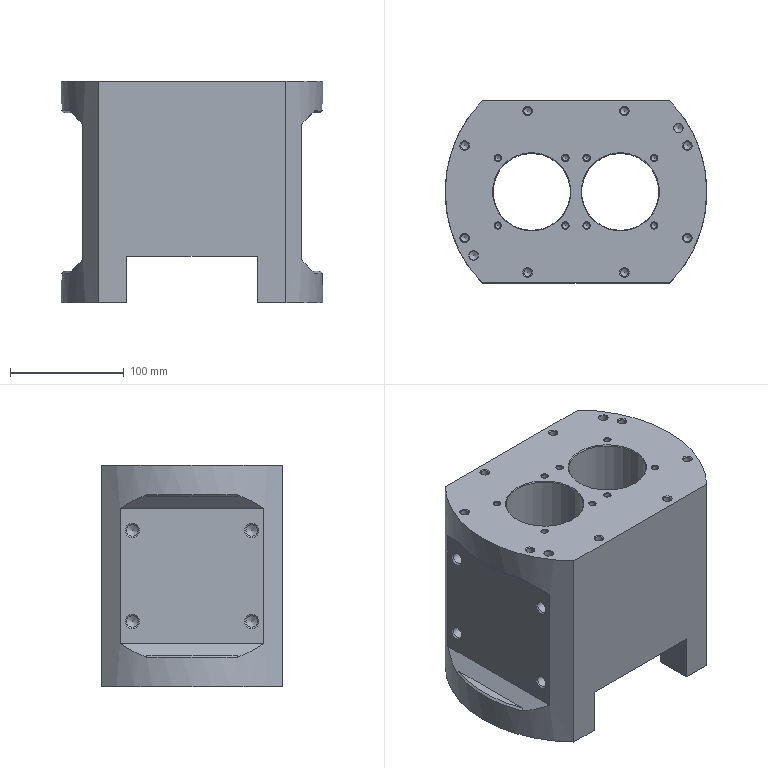CAM job | NX | 3+2 milling, drilling | part box 230 x 160 x 195 mm | stock box 230 x 230 x 195 mm
Tools:
number,name,description,diameter,corner_radius,flute_length,length,flutes
2,D50,Milling Tool-5 Parameters,50.0,0.0,50.0,75.0,2
1,ZXZ,Milling Tool-5 Parameters,6.0,0.0,50.0,75.0,2
11,10.2ZT,Drilling Tool,10.2,0.0,35.0,50.0,2
12,M12,Milling Tool-5 Parameters,10.2,0.0,30.0,30.0,4
7,D6A45,Milling Tool-5 Parameters,6.0,0.0,50.0,75.0,2
5,D6R0.5,Milling Tool-5 Parameters,6.0,0.5,50.0,75.0,2
10,D10,Milling Tool-5 Parameters,10.0,0.0,50.0,75.0,2
16,6.8ZT,Drilling Tool,6.8,0.0,35.0,50.0,2
18,M8,Milling Tool-5 Parameters,6.8,0.0,30.0,30.0,4
15,5.2ZT,Drilling Tool,5.0,0.0,35.0,50.0,2
14,M6,Milling Tool-5 Parameters,5.0,0.0,30.0,30.0,4
17,7.8ZT,Drilling Tool,7.8,0.0,35.0,50.0,2
18,8.0JD,Milling Tool-5 Parameters,8.0,0.0,30.0,30.0,4
19,11.8ZT,Drilling Tool,11.8,0.0,35.0,50.0,2
9,D35R.5,Milling Tool-5 Parameters,35.0,0.5,50.0,75.0,2
8,68.0JD,Milling Tool-5 Parameters,68.0,0.0,50.0,75.0,2
11,D10JING,Milling Tool-5 Parameters,10.0,0.0,50.0,75.0,2
20,8.5ZT,Drilling Tool,8.5,0.0,35.0,50.0,2
21,M10,Milling Tool-5 Parameters,8.5,0.0,30.0,30.0,4
22,12.0JD,Milling Tool-5 Parameters,12.0,0.0,30.0,30.0,4
Operations:
program,operation,operation_type,tool,method,geometry_group,spindle_rpm,surface_speed,feed_per_tooth,feed_cut,feed_plunge,cut_length_mm,path_length_mm,cut_time_min,machine_time_min
1,FLOOR_WALL,VolumeBased25DMillingOperation,D50,METHOD,A,1200.0,188.0,0.8333,2000.0,1000.0,131491.296,159721.141,66.046,68.869
1,FLOOR_WALL_COPY,VolumeBased25DMillingOperation,D50,METHOD,A,2500.0,392.0,0.2,1000.0,1000.0,1618.36,1742.36,1.618,1.631
1,DRILLING,Operation,ZXZ,METHOD,A,5000.0,94.0,0.025,250.0,0.0,16.0,436.155,0.064,0.106
1,DRILLING_COPY,Operation,10.2ZT,METHOD,A,1200.0,38.0,0.1042,250.0,0.0,128.258,660.67,0.513,0.5663
1,DRILLING_COPY_COPY,Operation,M12,METHOD,A,200.0,6.0,0.0022,1.75,0.0,116.0,636.155,66.286,66.338
1,PLANAR_MILL_COPY_COPY,PlanarMilling,D6A45,METHOD,A,7500.0,141.0,0.0833,1250.0,100.0,165.459,952.269,0.1324,0.211
2,FLOOR_WALL_COPY_1,VolumeBased25DMillingOperation,D50,METHOD,B,1200.0,188.0,0.8333,2000.0,1000.0,131491.296,159721.141,66.046,68.869
2,FLOOR_WALL_COPY_COPY,VolumeBased25DMillingOperation,D50,METHOD,B,2500.0,392.0,0.2,1000.0,1000.0,1618.36,1742.36,1.618,1.631
3,FLOOR_WALL_COPY_1_COPY,VolumeBased25DMillingOperation,D50,METHOD,C,1200.0,188.0,0.8333,2000.0,1000.0,26548.258,38956.342,13.436,14.677
3,FLOOR_WALL_COPY_COPY_COPY,VolumeBased25DMillingOperation,D50,METHOD,C,2500.0,392.0,0.2,1000.0,1000.0,610.897,702.897,0.6109,0.6201
3,ZLEVEL_PROFILE_COPY,ZLevelMilling,D10,METHOD,C,3500.0,109.0,0.3143,2200.0,1000.0,29490.997,29798.748,13.411,13.442
3,ZLEVEL_PROFILE,ZLevelMilling,D6R0.5,METHOD,C,6500.0,122.0,0.1923,2500.0,1000.0,48714.078,49006.867,19.491,19.52
3,DRILLING_COPY_1,Operation,ZXZ,METHOD,C,5000.0,94.0,0.025,250.0,0.0,16.0,404.155,0.064,0.1028
3,DRILLING_COPY_COPY_1,Operation,10.2ZT,METHOD,C,1200.0,38.0,0.1042,250.0,0.0,128.258,628.67,0.513,0.5631
3,DRILLING_COPY_COPY_COPY,Operation,M12,METHOD,C,200.0,6.0,0.0022,1.75,0.0,116.0,604.155,66.286,66.335
3,PLANAR_MILL_COPY_COPY_COPY,PlanarMilling,D6A45,METHOD,C,7500.0,141.0,0.0833,1250.0,100.0,165.459,808.437,0.1324,0.1967
4,FLOOR_WALL_COPY_1_COPY_COPY,VolumeBased25DMillingOperation,D50,METHOD,D,1200.0,188.0,0.8333,2000.0,1000.0,26548.258,38956.342,13.436,14.677
4,FLOOR_WALL_COPY_COPY_COPY_COPY,VolumeBased25DMillingOperation,D50,METHOD,D,2500.0,392.0,0.2,1000.0,1000.0,610.897,702.897,0.6109,0.6201
4,ZLEVEL_PROFILE_COPY_COPY,ZLevelMilling,D10,METHOD,D,3500.0,109.0,0.3143,2200.0,1000.0,29491.225,29798.895,13.411,13.442
4,ZLEVEL_PROFILE_COPY_1,ZLevelMilling,D6R0.5,METHOD,D,6500.0,122.0,0.1923,2500.0,1000.0,48719.87,49012.661,19.494,19.523
5,FLOOR_WALL_COPY_COPY_COPY_COPY_1,VolumeBased25DMillingOperation,D50,METHOD,E,2500.0,392.0,0.2,1000.0,1000.0,1462.804,1516.804,1.463,1.468
5,DRILLING_COPY_2,Operation,ZXZ,METHOD,E,5000.0,94.0,0.025,250.0,0.0,80.0,1015.001,0.32,0.4135
5,DRILLING_COPY_2_COPY,Operation,6.8ZT,METHOD,E,2000.0,42.0,0.05,200.0,0.0,240.343,1062.342,1.202,1.284
5,DRILLING_COPY_2_COPY_COPY,Operation,M8,METHOD,E,200.0,4.0,0.0016,1.25,0.0,224.0,1029.655,179.2,179.281
5,DRILLING_COPY_2_COPY_COPY_1,Operation,5.2ZT,METHOD,E,2000.0,42.0,0.05,200.0,0.0,196.017,808.085,0.9801,1.041
5,DRILLING_COPY_2_COPY_COPY_1_COPY,Operation,M6,METHOD,E,200.0,3.0,0.0013,1.0,0.0,184.0,784.05,184.0,184.06
5,DRILLING_COPY_2_COPY_COPY_1_COPY_1,Operation,7.8ZT,METHOD,E,2000.0,42.0,0.05,200.0,0.0,50.807,376.635,0.254,0.2866
5,DRILLING_COPY_2_COPY_COPY_1_COPY_1_COPY,Operation,8.0JD,METHOD,E,1000.0,25.0,0.01,40.0,0.0,46.0,367.021,1.15,1.182
5,DRILLING_COPY_COPY_1_COPY,Operation,11.8ZT,METHOD,E,1025.0,38.0,0.0732,150.0,0.0,323.09,788.206,2.154,2.2
5,HOLE_MILLING,CylinderMilling,D35R.5,METHOD,E,1500.0,164.0,0.4,1200.0,100.0,129337.553,129845.553,107.781,107.832
5,DRILLING_COPY_2_COPY_COPY_1_COPY_1_COPY_COPY,Operation,68.0JD,METHOD,E,300.0,64.0,0.0667,40.0,0.0,315.0,771.058,7.875,7.921
5,PLANAR_MILL_COPY_COPY_COPY_COPY,PlanarMilling,D6A45,METHOD,E,7500.0,141.0,0.0833,1250.0,100.0,870.393,2742.854,0.6963,0.8836
5,PLANAR_MILL_COPY_COPY_COPY_COPY_COPY,PlanarMilling,D6A45,METHOD,E,7500.0,141.0,0.0833,1250.0,100.0,702.422,759.422,0.5619,0.5676
6,FLOOR_WALL_COPY_COPY_COPY_COPY_1_COPY,VolumeBased25DMillingOperation,D50,METHOD,F,2500.0,392.0,0.2,1000.0,1000.0,1462.832,1516.832,1.463,1.468
6,FLOOR_WALL_1,VolumeBased25DMillingOperation,D50,METHOD,F,1200.0,188.0,0.8333,2000.0,1000.0,98987.376,105667.785,51.341,52.009
6,FLOOR_WALL_2_COPY,VolumeBased25DMillingOperation,D10JING,METHOD,F,5000.0,157.0,0.12,1200.0,500.0,3797.744,7374.744,3.291,3.648
6,FLOOR_WALL_2,VolumeBased25DMillingOperation,D10JING,METHOD,F,5000.0,157.0,0.12,1200.0,500.0,5135.729,5739.413,4.25,4.311
6,DRILLING_COPY_2_COPY_1,Operation,ZXZ,METHOD,F,5000.0,94.0,0.025,250.0,0.0,64.0,944.308,0.256,0.344
6,DRILLING_COPY_2_COPY_COPY_1_COPY_2,Operation,5.2ZT,METHOD,F,2000.0,42.0,0.05,200.0,0.0,196.017,890.085,0.9801,1.05
6,DRILLING_COPY_2_COPY_COPY_1_COPY_COPY,Operation,M6,METHOD,F,200.0,3.0,0.0013,1.0,0.0,184.0,866.05,184.0,184.068
6,DRILLING_COPY_2_COPY_COPY_1_COPY_2_COPY,Operation,8.5ZT,METHOD,F,2000.0,53.0,0.05,200.0,0.0,140.215,760.528,0.7011,0.7631
6,DRILLING_COPY_2_COPY_COPY_1_COPY_2_COPY_COPY,Operation,M10,METHOD,F,200.0,5.0,0.0019,1.5,0.0,130.0,740.098,86.667,86.728
6,DRILLING_COPY_2_COPY_COPY_1_COPY_1_COPY_1,Operation,11.8ZT,METHOD,F,2000.0,42.0,0.05,200.0,0.0,53.21,371.91,0.2661,0.2979
6,DRILLING_COPY_2_COPY_COPY_1_COPY_1_COPY_COPY_1,Operation,12.0JD,METHOD,F,1000.0,25.0,0.01,40.0,0.0,45.464,356.962,1.137,1.168
6,PLANAR_MILL_COPY_COPY_COPY_COPY_COPY_1,PlanarMilling,D6A45,METHOD,F,7500.0,141.0,0.0833,1250.0,100.0,215.384,991.021,0.1723,0.2499
6,PLANAR_MILL_COPY_COPY_COPY_COPY_COPY_1_COPY,PlanarMilling,D6A45,METHOD,F,7500.0,141.0,0.0833,1250.0,100.0,600.904,2402.514,0.4807,0.6609
6,PLANAR_MILL_COPY_COPY_COPY_COPY_COPY_COPY,PlanarMilling,D6A45,METHOD,F,7500.0,141.0,0.0833,1250.0,100.0,864.668,1088.668,0.6917,0.7141
6,PLANAR_MILL_COPY_COPY_COPY_COPY_COPY_COPY_COPY,PlanarMilling,D6A45,METHOD,F,7500.0,141.0,0.0833,1250.0,100.0,235.912,679.707,0.1887,0.2331